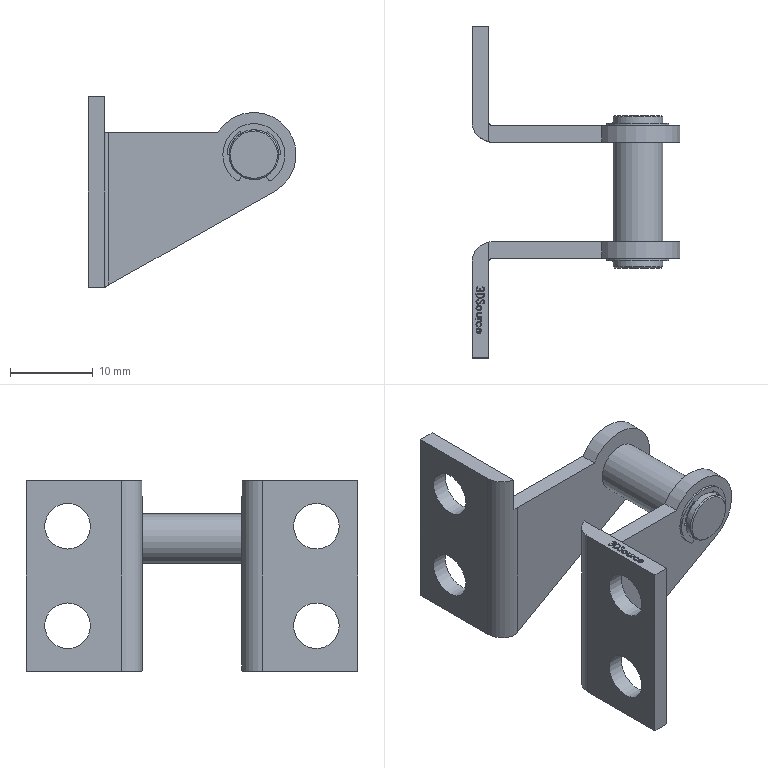Part | STEP file | 冲床-300配套压波_id694_x_t | 1 solid | 160 faces | box 25.1 x 40 x 23 mm | volume 2627 mm3 | plane 88 | cylinder 70 | cone 2 | commonest cylinder face diameters 0.2 x16 0.5 x8 5.4 x6 0.473 x5 0.379 x4 5.5 x4